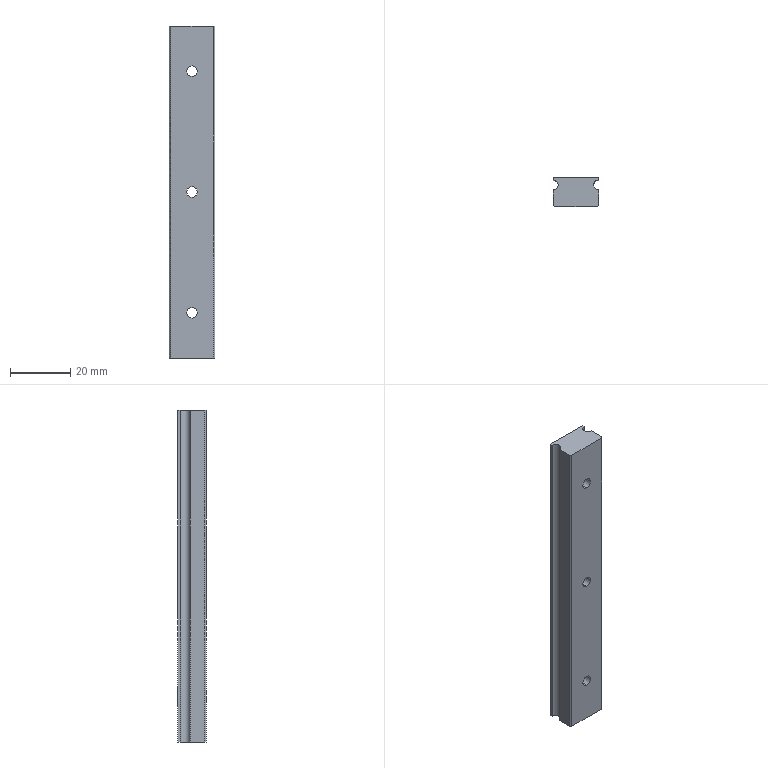Part | SolidWorks | features BaseBody 1 | 1 solid | 28 faces | box 15 x 9.5 x 110 mm | volume 14193 mm3 | cylinder 15 | plane 13 | commonest cylinder face diameters 3.5 x6 6 x6 3.28 x3
STEP:
#1=CARTESIAN_POINT('',(0.,9.5,58.));
#2=VERTEX_POINT('',#1);
#3=CARTESIAN_POINT('',(0.,9.5,52.));
#4=VERTEX_POINT('',#3);
#5=CARTESIAN_POINT('',(0.,9.5,55.));
#6=DIRECTION('',(0.,-1.,0.));
#7=DIRECTION('',(0.,0.,-1.));
#8=AXIS2_PLACEMENT_3D('',#5,#6,#7);
#9=CIRCLE('',#8,3.);
#10=EDGE_CURVE('',#2,#4,#9,.T.);
#11=ORIENTED_EDGE('',*,*,#10,.F.);
#12=CARTESIAN_POINT('',(0.,5.,58.));
#13=VERTEX_POINT('',#12);
#14=CARTESIAN_POINT('',(0.,7.25,58.));
#15=DIRECTION('',(0.,-1.,0.));
#16=VECTOR('',#15,1000.);
#17=LINE('',#14,#16);
#18=EDGE_CURVE('',#2,#13,#17,.T.);
#19=ORIENTED_EDGE('',*,*,#18,.T.);
#20=CARTESIAN_POINT('',(0.,5.,52.));
#21=VERTEX_POINT('',#20);
#22=CARTESIAN_POINT('',(0.,5.,55.));
#23=DIRECTION('',(0.,1.,0.));
#24=DIRECTION('',(0.,0.,-1.));
#25=AXIS2_PLACEMENT_3D('',#22,#23,#24);
#26=CIRCLE('',#25,3.);
#27=EDGE_CURVE('',#21,#13,#26,.T.);
#28=ORIENTED_EDGE('',*,*,#27,.F.);
#29=CARTESIAN_POINT('',(0.,7.25,52.));
#30=DIRECTION('',(0.,-1.,0.));
#31=VECTOR('',#30,1000.);
#32=LINE('',#29,#31);
#33=EDGE_CURVE('',#4,#21,#32,.T.);
#34=ORIENTED_EDGE('',*,*,#33,.F.);
#35=EDGE_LOOP('',(#11,#19,#28,#34));
#36=FACE_OUTER_BOUND('',#35,.T.);
#37=CARTESIAN_POINT('',(0.,7.25,55.));
#38=DIRECTION('',(0.,-1.,0.));
#39=DIRECTION('',(0.,0.,-1.));
#40=AXIS2_PLACEMENT_3D('',#37,#38,#39);
#41=CYLINDRICAL_SURFACE('',#40,3.);
#42=ADVANCED_FACE('',(#36),#41,.F.);
#43=CARTESIAN_POINT('',(0.,9.5,18.));
#44=VERTEX_POINT('',#43);
#45=CARTESIAN_POINT('',(0.,9.5,12.));
#46=VERTEX_POINT('',#45);
#47=CARTESIAN_POINT('',(0.,9.5,15.));
#48=DIRECTION('',(0.,-1.,0.));
#49=DIRECTION('',(0.,0.,-1.));
#50=AXIS2_PLACEMENT_3D('',#47,#48,#49);
#51=CIRCLE('',#50,3.);
#52=EDGE_CURVE('',#44,#46,#51,.T.);
#53=ORIENTED_EDGE('',*,*,#52,.F.);
#54=CARTESIAN_POINT('',(0.,5.,18.));
#55=VERTEX_POINT('',#54);
#56=CARTESIAN_POINT('',(0.,7.25,18.));
#57=DIRECTION('',(0.,-1.,0.));
#58=VECTOR('',#57,1000.);
#59=LINE('',#56,#58);
#60=EDGE_CURVE('',#44,#55,#59,.T.);
#61=ORIENTED_EDGE('',*,*,#60,.T.);
#62=CARTESIAN_POINT('',(0.,5.,12.));
#63=VERTEX_POINT('',#62);
#64=CARTESIAN_POINT('',(0.,5.,15.));
#65=DIRECTION('',(0.,1.,0.));
#66=DIRECTION('',(0.,0.,-1.));
#67=AXIS2_PLACEMENT_3D('',#64,#65,#66);
#68=CIRCLE('',#67,3.);
#69=EDGE_CURVE('',#63,#55,#68,.T.);
#70=ORIENTED_EDGE('',*,*,#69,.F.);
#71=CARTESIAN_POINT('',(0.,7.25,12.));
#72=DIRECTION('',(0.,-1.,0.));
#73=VECTOR('',#72,1000.);
#74=LINE('',#71,#73);
#75=EDGE_CURVE('',#46,#63,#74,.T.);
#76=ORIENTED_EDGE('',*,*,#75,.F.);
#77=EDGE_LOOP('',(#53,#61,#70,#76));
#78=FACE_OUTER_BOUND('',#77,.T.);
#79=CARTESIAN_POINT('',(0.,7.25,15.));
#80=DIRECTION('',(0.,-1.,0.));
#81=DIRECTION('',(0.,0.,-1.));
#82=AXIS2_PLACEMENT_3D('',#79,#80,#81);
#83=CYLINDRICAL_SURFACE('',#82,3.);
#84=ADVANCED_FACE('',(#78),#83,.F.);
#85=CARTESIAN_POINT('',(0.,9.5,98.));
#86=VERTEX_POINT('',#85);
#87=CARTESIAN_POINT('',(0.,9.5,92.));
#88=VERTEX_POINT('',#87);
#89=CARTESIAN_POINT('',(0.,9.5,95.));
#90=DIRECTION('',(0.,-1.,0.));
#91=DIRECTION('',(0.,0.,-1.));
#92=AXIS2_PLACEMENT_3D('',#89,#90,#91);
#93=CIRCLE('',#92,3.);
#94=EDGE_CURVE('',#86,#88,#93,.T.);
#95=ORIENTED_EDGE('',*,*,#94,.F.);
#96=CARTESIAN_POINT('',(0.,5.,98.));
#97=VERTEX_POINT('',#96);
#98=CARTESIAN_POINT('',(0.,7.25,98.));
#99=DIRECTION('',(0.,-1.,0.));
#100=VECTOR('',#99,1000.);
#101=LINE('',#98,#100);
#102=EDGE_CURVE('',#86,#97,#101,.T.);
#103=ORIENTED_EDGE('',*,*,#102,.T.);
#104=CARTESIAN_POINT('',(0.,5.,92.));
#105=VERTEX_POINT('',#104);
#106=CARTESIAN_POINT('',(0.,5.,95.));
#107=DIRECTION('',(0.,1.,0.));
#108=DIRECTION('',(0.,0.,-1.));
#109=AXIS2_PLACEMENT_3D('',#106,#107,#108);
#110=CIRCLE('',#109,3.);
#111=EDGE_CURVE('',#105,#97,#110,.T.);
#112=ORIENTED_EDGE('',*,*,#111,.F.);
#113=CARTESIAN_POINT('',(0.,7.25,92.));
#114=DIRECTION('',(0.,-1.,0.));
#115=VECTOR('',#114,1000.);
#116=LINE('',#113,#115);
#117=EDGE_CURVE('',#88,#105,#116,.T.);
#118=ORIENTED_EDGE('',*,*,#117,.F.);
#119=EDGE_LOOP('',(#95,#103,#112,#118));
#120=FACE_OUTER_BOUND('',#119,.T.);
#121=CARTESIAN_POINT('',(0.,7.25,95.));
#122=DIRECTION('',(0.,-1.,0.));
#123=DIRECTION('',(0.,0.,-1.));
#124=AXIS2_PLACEMENT_3D('',#121,#122,#123);
#125=CYLINDRICAL_SURFACE('',#124,3.);
#126=ADVANCED_FACE('',(#120),#125,.F.);
#127=CARTESIAN_POINT('',(5.86,7.02,110.));
#128=VERTEX_POINT('',#127);
#129=CARTESIAN_POINT('',(7.5,8.66,110.));
#130=VERTEX_POINT('',#129);
#131=CARTESIAN_POINT('',(7.5,7.02,110.));
#132=DIRECTION('',(0.,0.,-1.));
#133=DIRECTION('',(-1.,0.,0.));
#134=AXIS2_PLACEMENT_3D('',#131,#132,#133);
#135=CIRCLE('',#134,1.64);
#136=EDGE_CURVE('',#128,#130,#135,.T.);
#137=ORIENTED_EDGE('',*,*,#136,.F.);
#138=CARTESIAN_POINT('',(5.86,7.02,0.));
#139=VERTEX_POINT('',#138);
#140=CARTESIAN_POINT('',(5.86,7.02,0.));
#141=DIRECTION('',(0.,0.,-1.));
#142=VECTOR('',#141,1000.);
#143=LINE('',#140,#142);
#144=EDGE_CURVE('',#128,#139,#143,.T.);
#145=ORIENTED_EDGE('',*,*,#144,.T.);
#146=CARTESIAN_POINT('',(7.5,8.66,0.));
#147=VERTEX_POINT('',#146);
#148=CARTESIAN_POINT('',(7.5,7.02,0.));
#149=DIRECTION('',(0.,0.,-1.));
#150=DIRECTION('',(-1.,0.,0.));
#151=AXIS2_PLACEMENT_3D('',#148,#149,#150);
#152=CIRCLE('',#151,1.64);
#153=EDGE_CURVE('',#139,#147,#152,.T.);
#154=ORIENTED_EDGE('',*,*,#153,.T.);
#155=CARTESIAN_POINT('',(7.5,8.66,0.));
#156=DIRECTION('',(0.,0.,-1.));
#157=VECTOR('',#156,1000.);
#158=LINE('',#155,#157);
#159=EDGE_CURVE('',#130,#147,#158,.T.);
#160=ORIENTED_EDGE('',*,*,#159,.F.);
#161=EDGE_LOOP('',(#137,#145,#154,#160));
#162=FACE_OUTER_BOUND('',#161,.T.);
#163=CARTESIAN_POINT('',(7.5,7.02,0.));
#164=DIRECTION('',(0.,0.,-1.));
#165=DIRECTION('',(-1.,0.,0.));
#166=AXIS2_PLACEMENT_3D('',#163,#164,#165);
#167=CYLINDRICAL_SURFACE('',#166,1.64);
#168=ADVANCED_FACE('',(#162),#167,.F.);
#169=CARTESIAN_POINT('',(0.,5.,53.25));
#170=VERTEX_POINT('',#169);
#171=CARTESIAN_POINT('',(0.,5.,56.75));
#172=VERTEX_POINT('',#171);
#173=CARTESIAN_POINT('',(0.,5.,55.));
#174=DIRECTION('',(0.,1.,0.));
#175=DIRECTION('',(0.,0.,-1.));
#176=AXIS2_PLACEMENT_3D('',#173,#174,#175);
#177=CIRCLE('',#176,1.75);
#178=EDGE_CURVE('',#170,#172,#177,.T.);
#179=ORIENTED_EDGE('',*,*,#178,.T.);
#180=CARTESIAN_POINT('',(0.,0.,56.75));
#181=VERTEX_POINT('',#180);
#182=CARTESIAN_POINT('',(0.,2.5,56.75));
#183=DIRECTION('',(0.,-1.,0.));
#184=VECTOR('',#183,1000.);
#185=LINE('',#182,#184);
#186=EDGE_CURVE('',#172,#181,#185,.T.);
#187=ORIENTED_EDGE('',*,*,#186,.T.);
#188=CARTESIAN_POINT('',(0.,0.,53.25));
#189=VERTEX_POINT('',#188);
#190=CARTESIAN_POINT('',(0.,0.,55.));
#191=DIRECTION('',(0.,1.,0.));
#192=DIRECTION('',(0.,0.,-1.));
#193=AXIS2_PLACEMENT_3D('',#190,#191,#192);
#194=CIRCLE('',#193,1.75);
#195=EDGE_CURVE('',#189,#181,#194,.T.);
#196=ORIENTED_EDGE('',*,*,#195,.F.);
#197=CARTESIAN_POINT('',(0.,2.5,53.25));
#198=DIRECTION('',(0.,-1.,0.));
#199=VECTOR('',#198,1000.);
#200=LINE('',#197,#199);
#201=EDGE_CURVE('',#170,#189,#200,.T.);
#202=ORIENTED_EDGE('',*,*,#201,.F.);
#203=EDGE_LOOP('',(#179,#187,#196,#202));
#204=FACE_OUTER_BOUND('',#203,.T.);
#205=CARTESIAN_POINT('',(0.,2.5,55.));
#206=DIRECTION('',(0.,-1.,0.));
#207=DIRECTION('',(0.,0.,-1.));
#208=AXIS2_PLACEMENT_3D('',#205,#206,#207);
#209=CYLINDRICAL_SURFACE('',#208,1.75);
#210=ADVANCED_FACE('',(#204),#209,.F.);
#211=CARTESIAN_POINT('',(0.,5.,13.25));
#212=VERTEX_POINT('',#211);
#213=CARTESIAN_POINT('',(0.,5.,16.75));
#214=VERTEX_POINT('',#213);
#215=CARTESIAN_POINT('',(0.,5.,15.));
#216=DIRECTION('',(0.,1.,0.));
#217=DIRECTION('',(0.,0.,-1.));
#218=AXIS2_PLACEMENT_3D('',#215,#216,#217);
#219=CIRCLE('',#218,1.75);
#220=EDGE_CURVE('',#212,#214,#219,.T.);
#221=ORIENTED_EDGE('',*,*,#220,.T.);
#222=CARTESIAN_POINT('',(0.,0.,16.75));
#223=VERTEX_POINT('',#222);
#224=CARTESIAN_POINT('',(0.,2.5,16.75));
#225=DIRECTION('',(0.,-1.,0.));
#226=VECTOR('',#225,1000.);
#227=LINE('',#224,#226);
#228=EDGE_CURVE('',#214,#223,#227,.T.);
#229=ORIENTED_EDGE('',*,*,#228,.T.);
#230=CARTESIAN_POINT('',(0.,0.,13.25));
#231=VERTEX_POINT('',#230);
#232=CARTESIAN_POINT('',(0.,0.,15.));
#233=DIRECTION('',(0.,1.,0.));
#234=DIRECTION('',(0.,0.,-1.));
#235=AXIS2_PLACEMENT_3D('',#232,#233,#234);
#236=CIRCLE('',#235,1.75);
#237=EDGE_CURVE('',#231,#223,#236,.T.);
#238=ORIENTED_EDGE('',*,*,#237,.F.);
#239=CARTESIAN_POINT('',(0.,2.5,13.25));
#240=DIRECTION('',(0.,-1.,0.));
#241=VECTOR('',#240,1000.);
#242=LINE('',#239,#241);
#243=EDGE_CURVE('',#212,#231,#242,.T.);
#244=ORIENTED_EDGE('',*,*,#243,.F.);
#245=EDGE_LOOP('',(#221,#229,#238,#244));
#246=FACE_OUTER_BOUND('',#245,.T.);
#247=CARTESIAN_POINT('',(0.,2.5,15.));
#248=DIRECTION('',(0.,-1.,0.));
#249=DIRECTION('',(0.,0.,-1.));
#250=AXIS2_PLACEMENT_3D('',#247,#248,#249);
#251=CYLINDRICAL_SURFACE('',#250,1.75);
#252=ADVANCED_FACE('',(#246),#251,.F.);
#253=CARTESIAN_POINT('',(0.,5.,93.25));
#254=VERTEX_POINT('',#253);
#255=CARTESIAN_POINT('',(0.,5.,96.75));
#256=VERTEX_POINT('',#255);
#257=CARTESIAN_POINT('',(0.,5.,95.));
#258=DIRECTION('',(0.,1.,0.));
#259=DIRECTION('',(0.,0.,-1.));
#260=AXIS2_PLACEMENT_3D('',#257,#258,#259);
#261=CIRCLE('',#260,1.75);
#262=EDGE_CURVE('',#254,#256,#261,.T.);
#263=ORIENTED_EDGE('',*,*,#262,.T.);
#264=CARTESIAN_POINT('',(0.,0.,96.75));
#265=VERTEX_POINT('',#264);
#266=CARTESIAN_POINT('',(0.,2.5,96.75));
#267=DIRECTION('',(0.,-1.,0.));
#268=VECTOR('',#267,1000.);
#269=LINE('',#266,#268);
#270=EDGE_CURVE('',#256,#265,#269,.T.);
#271=ORIENTED_EDGE('',*,*,#270,.T.);
#272=CARTESIAN_POINT('',(0.,0.,93.25));
#273=VERTEX_POINT('',#272);
#274=CARTESIAN_POINT('',(0.,0.,95.));
#275=DIRECTION('',(0.,1.,0.));
#276=DIRECTION('',(0.,0.,-1.));
#277=AXIS2_PLACEMENT_3D('',#274,#275,#276);
#278=CIRCLE('',#277,1.75);
#279=EDGE_CURVE('',#273,#265,#278,.T.);
#280=ORIENTED_EDGE('',*,*,#279,.F.);
#281=CARTESIAN_POINT('',(0.,2.5,93.25));
#282=DIRECTION('',(0.,-1.,0.));
#283=VECTOR('',#282,1000.);
#284=LINE('',#281,#283);
#285=EDGE_CURVE('',#254,#273,#284,.T.);
#286=ORIENTED_EDGE('',*,*,#285,.F.);
#287=EDGE_LOOP('',(#263,#271,#280,#286));
#288=FACE_OUTER_BOUND('',#287,.T.);
#289=CARTESIAN_POINT('',(0.,2.5,95.));
#290=DIRECTION('',(0.,-1.,0.));
#291=DIRECTION('',(0.,0.,-1.));
#292=AXIS2_PLACEMENT_3D('',#289,#290,#291);
#293=CYLINDRICAL_SURFACE('',#292,1.75);
#294=ADVANCED_FACE('',(#288),#293,.F.);
#295=CARTESIAN_POINT('',(0.,9.5,55.));
#296=DIRECTION('',(0.,-1.,0.));
#297=DIRECTION('',(0.,0.,-1.));
#298=AXIS2_PLACEMENT_3D('',#295,#296,#297);
#299=CIRCLE('',#298,3.);
#300=EDGE_CURVE('',#4,#2,#299,.T.);
#301=ORIENTED_EDGE('',*,*,#300,.T.);
#302=ORIENTED_EDGE('',*,*,#10,.T.);
#303=EDGE_LOOP('',(#301,#302));
#304=FACE_BOUND('',#303,.T.);
#305=CARTESIAN_POINT('',(0.,9.5,15.));
#306=DIRECTION('',(0.,-1.,0.));
#307=DIRECTION('',(0.,0.,-1.));
#308=AXIS2_PLACEMENT_3D('',#305,#306,#307);
#309=CIRCLE('',#308,3.);
#310=EDGE_CURVE('',#46,#44,#309,.T.);
#311=ORIENTED_EDGE('',*,*,#310,.T.);
#312=ORIENTED_EDGE('',*,*,#52,.T.);
#313=EDGE_LOOP('',(#311,#312));
#314=FACE_BOUND('',#313,.T.);
#315=CARTESIAN_POINT('',(0.,9.5,95.));
#316=DIRECTION('',(0.,-1.,0.));
#317=DIRECTION('',(0.,0.,-1.));
#318=AXIS2_PLACEMENT_3D('',#315,#316,#317);
#319=CIRCLE('',#318,3.);
#320=EDGE_CURVE('',#88,#86,#319,.T.);
#321=ORIENTED_EDGE('',*,*,#320,.T.);
#322=ORIENTED_EDGE('',*,*,#94,.T.);
#323=EDGE_LOOP('',(#321,#322));
#324=FACE_BOUND('',#323,.T.);
#325=CARTESIAN_POINT('',(7.5,9.5,0.));
#326=VERTEX_POINT('',#325);
#327=CARTESIAN_POINT('',(-7.5,9.5,0.));
#328=VERTEX_POINT('',#327);
#329=CARTESIAN_POINT('',(-7.5,9.5,0.));
#330=DIRECTION('',(-1.,0.,0.));
#331=VECTOR('',#330,1000.);
#332=LINE('',#329,#331);
#333=EDGE_CURVE('',#326,#328,#332,.T.);
#334=ORIENTED_EDGE('',*,*,#333,.T.);
#335=CARTESIAN_POINT('',(-7.5,9.5,110.));
#336=VERTEX_POINT('',#335);
#337=CARTESIAN_POINT('',(-7.5,9.5,0.));
#338=DIRECTION('',(0.,0.,1.));
#339=VECTOR('',#338,1000.);
#340=LINE('',#337,#339);
#341=EDGE_CURVE('',#328,#336,#340,.T.);
#342=ORIENTED_EDGE('',*,*,#341,.T.);
#343=CARTESIAN_POINT('',(7.5,9.5,110.));
#344=VERTEX_POINT('',#343);
#345=CARTESIAN_POINT('',(-7.5,9.5,110.));
#346=DIRECTION('',(1.,0.,0.));
#347=VECTOR('',#346,1000.);
#348=LINE('',#345,#347);
#349=EDGE_CURVE('',#336,#344,#348,.T.);
#350=ORIENTED_EDGE('',*,*,#349,.T.);
#351=CARTESIAN_POINT('',(7.5,9.5,0.));
#352=DIRECTION('',(0.,0.,-1.));
#353=VECTOR('',#352,1000.);
#354=LINE('',#351,#353);
#355=EDGE_CURVE('',#344,#326,#354,.T.);
#356=ORIENTED_EDGE('',*,*,#355,.T.);
#357=EDGE_LOOP('',(#334,#342,#350,#356));
#358=FACE_OUTER_BOUND('',#357,.T.);
#359=CARTESIAN_POINT('',(-7.5,9.5,0.));
#360=DIRECTION('',(0.,1.,0.));
#361=DIRECTION('',(0.,0.,1.));
#362=AXIS2_PLACEMENT_3D('',#359,#360,#361);
#363=PLANE('',#362);
#364=ADVANCED_FACE('',(#304,#314,#324,#358),#363,.T.);
#365=ORIENTED_EDGE('',*,*,#18,.F.);
#366=ORIENTED_EDGE('',*,*,#300,.F.);
#367=ORIENTED_EDGE('',*,*,#33,.T.);
#368=CARTESIAN_POINT('',(0.,5.,55.));
#369=DIRECTION('',(0.,1.,0.));
#370=DIRECTION('',(0.,0.,-1.));
#371=AXIS2_PLACEMENT_3D('',#368,#369,#370);
#372=CIRCLE('',#371,3.);
#373=EDGE_CURVE('',#13,#21,#372,.T.);
#374=ORIENTED_EDGE('',*,*,#373,.F.);
#375=EDGE_LOOP('',(#365,#366,#367,#374));
#376=FACE_OUTER_BOUND('',#375,.T.);
#377=CARTESIAN_POINT('',(0.,7.25,55.));
#378=DIRECTION('',(0.,-1.,0.));
#379=DIRECTION('',(0.,0.,-1.));
#380=AXIS2_PLACEMENT_3D('',#377,#378,#379);
#381=CYLINDRICAL_SURFACE('',#380,3.);
#382=ADVANCED_FACE('',(#376),#381,.F.);
#383=ORIENTED_EDGE('',*,*,#60,.F.);
#384=ORIENTED_EDGE('',*,*,#310,.F.);
#385=ORIENTED_EDGE('',*,*,#75,.T.);
#386=CARTESIAN_POINT('',(0.,5.,15.));
#387=DIRECTION('',(0.,1.,0.));
#388=DIRECTION('',(0.,0.,-1.));
#389=AXIS2_PLACEMENT_3D('',#386,#387,#388);
#390=CIRCLE('',#389,3.);
#391=EDGE_CURVE('',#55,#63,#390,.T.);
#392=ORIENTED_EDGE('',*,*,#391,.F.);
#393=EDGE_LOOP('',(#383,#384,#385,#392));
#394=FACE_OUTER_BOUND('',#393,.T.);
#395=CARTESIAN_POINT('',(0.,7.25,15.));
#396=DIRECTION('',(0.,-1.,0.));
#397=DIRECTION('',(0.,0.,-1.));
#398=AXIS2_PLACEMENT_3D('',#395,#396,#397);
#399=CYLINDRICAL_SURFACE('',#398,3.);
#400=ADVANCED_FACE('',(#394),#399,.F.);
#401=ORIENTED_EDGE('',*,*,#102,.F.);
#402=ORIENTED_EDGE('',*,*,#320,.F.);
#403=ORIENTED_EDGE('',*,*,#117,.T.);
#404=CARTESIAN_POINT('',(0.,5.,95.));
#405=DIRECTION('',(0.,1.,0.));
#406=DIRECTION('',(0.,0.,-1.));
#407=AXIS2_PLACEMENT_3D('',#404,#405,#406);
#408=CIRCLE('',#407,3.);
#409=EDGE_CURVE('',#97,#105,#408,.T.);
#410=ORIENTED_EDGE('',*,*,#409,.F.);
#411=EDGE_LOOP('',(#401,#402,#403,#410));
#412=FACE_OUTER_BOUND('',#411,.T.);
#413=CARTESIAN_POINT('',(0.,7.25,95.));
#414=DIRECTION('',(0.,-1.,0.));
#415=DIRECTION('',(0.,0.,-1.));
#416=AXIS2_PLACEMENT_3D('',#413,#414,#415);
#417=CYLINDRICAL_SURFACE('',#416,3.);
#418=ADVANCED_FACE('',(#412),#417,.F.);
#419=CARTESIAN_POINT('',(-7.5,8.66,0.));
#420=VERTEX_POINT('',#419);
#421=CARTESIAN_POINT('',(-7.5,8.66,0.));
#422=DIRECTION('',(0.,-1.,0.));
#423=VECTOR('',#422,1000.);
#424=LINE('',#421,#423);
#425=EDGE_CURVE('',#328,#420,#424,.T.);
#426=ORIENTED_EDGE('',*,*,#425,.T.);
#427=CARTESIAN_POINT('',(-7.5,8.66,110.));
#428=VERTEX_POINT('',#427);
#429=CARTESIAN_POINT('',(-7.5,8.66,0.));
#430=DIRECTION('',(0.,0.,1.));
#431=VECTOR('',#430,1000.);
#432=LINE('',#429,#431);
#433=EDGE_CURVE('',#420,#428,#432,.T.);
#434=ORIENTED_EDGE('',*,*,#433,.T.);
#435=CARTESIAN_POINT('',(-7.5,8.66,110.));
#436=DIRECTION('',(0.,1.,0.));
#437=VECTOR('',#436,1000.);
#438=LINE('',#435,#437);
#439=EDGE_CURVE('',#428,#336,#438,.T.);
#440=ORIENTED_EDGE('',*,*,#439,.T.);
#441=ORIENTED_EDGE('',*,*,#341,.F.);
#442=EDGE_LOOP('',(#426,#434,#440,#441));
#443=FACE_OUTER_BOUND('',#442,.T.);
#444=CARTESIAN_POINT('',(-7.5,8.66,0.));
#445=DIRECTION('',(-1.,0.,0.));
#446=DIRECTION('',(0.,0.,1.));
#447=AXIS2_PLACEMENT_3D('',#444,#445,#446);
#448=PLANE('',#447);
#449=ADVANCED_FACE('',(#443),#448,.T.);
#450=ORIENTED_EDGE('',*,*,#333,.F.);
#451=CARTESIAN_POINT('',(7.5,0.,0.));
#452=DIRECTION('',(0.,1.,0.));
#453=VECTOR('',#452,1000.);
#454=LINE('',#451,#453);
#455=EDGE_CURVE('',#147,#326,#454,.T.);
#456=ORIENTED_EDGE('',*,*,#455,.F.);
#457=ORIENTED_EDGE('',*,*,#153,.F.);
#458=CARTESIAN_POINT('',(7.5,5.38,0.));
#459=VERTEX_POINT('',#458);
#460=CARTESIAN_POINT('',(7.5,7.02,0.));
#461=DIRECTION('',(0.,0.,-1.));
#462=DIRECTION('',(-1.,0.,0.));
#463=AXIS2_PLACEMENT_3D('',#460,#461,#462);
#464=CIRCLE('',#463,1.64);
#465=EDGE_CURVE('',#459,#139,#464,.T.);
#466=ORIENTED_EDGE('',*,*,#465,.F.);
#467=CARTESIAN_POINT('',(7.5,0.495,0.));
#468=VERTEX_POINT('',#467);
#469=CARTESIAN_POINT('',(7.5,0.,0.));
#470=DIRECTION('',(0.,1.,0.));
#471=VECTOR('',#470,1000.);
#472=LINE('',#469,#471);
#473=EDGE_CURVE('',#468,#459,#472,.T.);
#474=ORIENTED_EDGE('',*,*,#473,.F.);
#475=CARTESIAN_POINT('',(7.005,0.,0.));
#476=VERTEX_POINT('',#475);
#477=CARTESIAN_POINT('',(7.5,0.495,0.));
#478=DIRECTION('',(0.7071,0.7071,0.));
#479=VECTOR('',#478,1000.);
#480=LINE('',#477,#479);
#481=EDGE_CURVE('',#476,#468,#480,.T.);
#482=ORIENTED_EDGE('',*,*,#481,.F.);
#483=CARTESIAN_POINT('',(-7.005,0.,0.));
#484=VERTEX_POINT('',#483);
#485=CARTESIAN_POINT('',(0.,0.,0.));
#486=DIRECTION('',(1.,0.,0.));
#487=VECTOR('',#486,1000.);
#488=LINE('',#485,#487);
#489=EDGE_CURVE('',#484,#476,#488,.T.);
#490=ORIENTED_EDGE('',*,*,#489,.F.);
#491=CARTESIAN_POINT('',(-7.5,0.495,0.));
#492=VERTEX_POINT('',#491);
#493=CARTESIAN_POINT('',(-7.005,0.,0.));
#494=DIRECTION('',(0.7071,-0.7071,0.));
#495=VECTOR('',#494,1000.);
#496=LINE('',#493,#495);
#497=EDGE_CURVE('',#492,#484,#496,.T.);
#498=ORIENTED_EDGE('',*,*,#497,.F.);
#499=CARTESIAN_POINT('',(-7.5,5.38,0.));
#500=VERTEX_POINT('',#499);
#501=CARTESIAN_POINT('',(-7.5,0.,0.));
#502=DIRECTION('',(0.,-1.,0.));
#503=VECTOR('',#502,1000.);
#504=LINE('',#501,#503);
#505=EDGE_CURVE('',#500,#492,#504,.T.);
#506=ORIENTED_EDGE('',*,*,#505,.F.);
#507=CARTESIAN_POINT('',(-7.5,7.02,0.));
#508=DIRECTION('',(0.,0.,-1.));
#509=DIRECTION('',(-1.,0.,0.));
#510=AXIS2_PLACEMENT_3D('',#507,#508,#509);
#511=CIRCLE('',#510,1.64);
#512=EDGE_CURVE('',#420,#500,#511,.T.);
#513=ORIENTED_EDGE('',*,*,#512,.F.);
#514=ORIENTED_EDGE('',*,*,#425,.F.);
#515=EDGE_LOOP('',(#450,#456,#457,#466,#474,#482,#490,#498,#506,#513,#514));
#516=FACE_OUTER_BOUND('',#515,.T.);
#517=CARTESIAN_POINT('',(0.,0.,0.));
#518=DIRECTION('',(0.,0.,1.));
#519=DIRECTION('',(1.,0.,0.));
#520=AXIS2_PLACEMENT_3D('',#517,#518,#519);
#521=PLANE('',#520);
#522=ADVANCED_FACE('',(#516),#521,.F.);
#523=ORIENTED_EDGE('',*,*,#455,.T.);
#524=ORIENTED_EDGE('',*,*,#355,.F.);
#525=CARTESIAN_POINT('',(7.5,9.5,110.));
#526=DIRECTION('',(0.,-1.,0.));
#527=VECTOR('',#526,1000.);
#528=LINE('',#525,#527);
#529=EDGE_CURVE('',#344,#130,#528,.T.);
#530=ORIENTED_EDGE('',*,*,#529,.T.);
#531=ORIENTED_EDGE('',*,*,#159,.T.);
#532=EDGE_LOOP('',(#523,#524,#530,#531));
#533=FACE_OUTER_BOUND('',#532,.T.);
#534=CARTESIAN_POINT('',(7.5,9.5,0.));
#535=DIRECTION('',(1.,0.,0.));
#536=DIRECTION('',(0.,0.,-1.));
#537=AXIS2_PLACEMENT_3D('',#534,#535,#536);
#538=PLANE('',#537);
#539=ADVANCED_FACE('',(#533),#538,.T.);
#540=CARTESIAN_POINT('',(7.5,5.38,110.));
#541=VERTEX_POINT('',#540);
#542=CARTESIAN_POINT('',(7.5,7.02,110.));
#543=DIRECTION('',(0.,0.,-1.));
#544=DIRECTION('',(-1.,0.,0.));
#545=AXIS2_PLACEMENT_3D('',#542,#543,#544);
#546=CIRCLE('',#545,1.64);
#547=EDGE_CURVE('',#541,#128,#546,.T.);
#548=ORIENTED_EDGE('',*,*,#547,.T.);
#549=ORIENTED_EDGE('',*,*,#136,.T.);
#550=ORIENTED_EDGE('',*,*,#529,.F.);
#551=ORIENTED_EDGE('',*,*,#349,.F.);
#552=ORIENTED_EDGE('',*,*,#439,.F.);
#553=CARTESIAN_POINT('',(-7.5,5.38,110.));
#554=VERTEX_POINT('',#553);
#555=CARTESIAN_POINT('',(-7.5,7.02,110.));
#556=DIRECTION('',(0.,0.,-1.));
#557=DIRECTION('',(-1.,0.,0.));
#558=AXIS2_PLACEMENT_3D('',#555,#556,#557);
#559=CIRCLE('',#558,1.64);
#560=EDGE_CURVE('',#428,#554,#559,.T.);
#561=ORIENTED_EDGE('',*,*,#560,.T.);
#562=CARTESIAN_POINT('',(-7.5,0.495,110.));
#563=VERTEX_POINT('',#562);
#564=CARTESIAN_POINT('',(-7.5,0.,110.));
#565=DIRECTION('',(0.,-1.,0.));
#566=VECTOR('',#565,1000.);
#567=LINE('',#564,#566);
#568=EDGE_CURVE('',#554,#563,#567,.T.);
#569=ORIENTED_EDGE('',*,*,#568,.T.);
#570=CARTESIAN_POINT('',(-7.005,0.,110.));
#571=VERTEX_POINT('',#570);
#572=CARTESIAN_POINT('',(-7.005,0.,110.));
#573=DIRECTION('',(-0.7071,0.7071,0.));
#574=VECTOR('',#573,1000.);
#575=LINE('',#572,#574);
#576=EDGE_CURVE('',#571,#563,#575,.T.);
#577=ORIENTED_EDGE('',*,*,#576,.F.);
#578=CARTESIAN_POINT('',(7.005,0.,110.));
#579=VERTEX_POINT('',#578);
#580=CARTESIAN_POINT('',(0.,0.,110.));
#581=DIRECTION('',(1.,0.,0.));
#582=VECTOR('',#581,1000.);
#583=LINE('',#580,#582);
#584=EDGE_CURVE('',#571,#579,#583,.T.);
#585=ORIENTED_EDGE('',*,*,#584,.T.);
#586=CARTESIAN_POINT('',(7.5,0.495,110.));
#587=VERTEX_POINT('',#586);
#588=CARTESIAN_POINT('',(7.5,0.495,110.));
#589=DIRECTION('',(-0.7071,-0.7071,0.));
#590=VECTOR('',#589,1000.);
#591=LINE('',#588,#590);
#592=EDGE_CURVE('',#587,#579,#591,.T.);
#593=ORIENTED_EDGE('',*,*,#592,.F.);
#594=CARTESIAN_POINT('',(7.5,0.,110.));
#595=DIRECTION('',(0.,1.,0.));
#596=VECTOR('',#595,1000.);
#597=LINE('',#594,#596);
#598=EDGE_CURVE('',#587,#541,#597,.T.);
#599=ORIENTED_EDGE('',*,*,#598,.T.);
#600=EDGE_LOOP('',(#548,#549,#550,#551,#552,#561,#569,#577,#585,#593,#599));
#601=FACE_OUTER_BOUND('',#600,.T.);
#602=CARTESIAN_POINT('',(0.,0.,110.));
#603=DIRECTION('',(0.,0.,1.));
#604=DIRECTION('',(1.,0.,0.));
#605=AXIS2_PLACEMENT_3D('',#602,#603,#604);
#606=PLANE('',#605);
#607=ADVANCED_FACE('',(#601),#606,.T.);
#608=ORIENTED_EDGE('',*,*,#178,.F.);
#609=CARTESIAN_POINT('',(0.,5.,55.));
#610=DIRECTION('',(0.,1.,0.));
#611=DIRECTION('',(0.,0.,-1.));
#612=AXIS2_PLACEMENT_3D('',#609,#610,#611);
#613=CIRCLE('',#612,1.75);
#614=EDGE_CURVE('',#172,#170,#613,.T.);
#615=ORIENTED_EDGE('',*,*,#614,.F.);
#616=EDGE_LOOP('',(#608,#615));
#617=FACE_BOUND('',#616,.T.);
#618=ORIENTED_EDGE('',*,*,#27,.T.);
#619=ORIENTED_EDGE('',*,*,#373,.T.);
#620=EDGE_LOOP('',(#618,#619));
#621=FACE_OUTER_BOUND('',#620,.T.);
#622=CARTESIAN_POINT('',(0.,5.,52.625));
#623=DIRECTION('',(0.,-1.,0.));
#624=DIRECTION('',(0.,0.,-1.));
#625=AXIS2_PLACEMENT_3D('',#622,#623,#624);
#626=PLANE('',#625);
#627=ADVANCED_FACE('',(#617,#621),#626,.F.);
#628=ORIENTED_EDGE('',*,*,#220,.F.);
#629=CARTESIAN_POINT('',(0.,5.,15.));
#630=DIRECTION('',(0.,1.,0.));
#631=DIRECTION('',(0.,0.,-1.));
#632=AXIS2_PLACEMENT_3D('',#629,#630,#631);
#633=CIRCLE('',#632,1.75);
#634=EDGE_CURVE('',#214,#212,#633,.T.);
#635=ORIENTED_EDGE('',*,*,#634,.F.);
#636=EDGE_LOOP('',(#628,#635));
#637=FACE_BOUND('',#636,.T.);
#638=ORIENTED_EDGE('',*,*,#69,.T.);
#639=ORIENTED_EDGE('',*,*,#391,.T.);
#640=EDGE_LOOP('',(#638,#639));
#641=FACE_OUTER_BOUND('',#640,.T.);
#642=CARTESIAN_POINT('',(0.,5.,12.625));
#643=DIRECTION('',(0.,-1.,0.));
#644=DIRECTION('',(0.,0.,-1.));
#645=AXIS2_PLACEMENT_3D('',#642,#643,#644);
#646=PLANE('',#645);
#647=ADVANCED_FACE('',(#637,#641),#646,.F.);
#648=ORIENTED_EDGE('',*,*,#262,.F.);
#649=CARTESIAN_POINT('',(0.,5.,95.));
#650=DIRECTION('',(0.,1.,0.));
#651=DIRECTION('',(0.,0.,-1.));
#652=AXIS2_PLACEMENT_3D('',#649,#650,#651);
#653=CIRCLE('',#652,1.75);
#654=EDGE_CURVE('',#256,#254,#653,.T.);
#655=ORIENTED_EDGE('',*,*,#654,.F.);
#656=EDGE_LOOP('',(#648,#655));
#657=FACE_BOUND('',#656,.T.);
#658=ORIENTED_EDGE('',*,*,#111,.T.);
#659=ORIENTED_EDGE('',*,*,#409,.T.);
#660=EDGE_LOOP('',(#658,#659));
#661=FACE_OUTER_BOUND('',#660,.T.);
#662=CARTESIAN_POINT('',(0.,5.,92.625));
#663=DIRECTION('',(0.,-1.,0.));
#664=DIRECTION('',(0.,0.,-1.));
#665=AXIS2_PLACEMENT_3D('',#662,#663,#664);
#666=PLANE('',#665);
#667=ADVANCED_FACE('',(#657,#661),#666,.F.);
#668=ORIENTED_EDGE('',*,*,#433,.F.);
#669=ORIENTED_EDGE('',*,*,#512,.T.);
#670=CARTESIAN_POINT('',(-7.5,5.38,0.));
#671=DIRECTION('',(0.,0.,-1.));
#672=VECTOR('',#671,1000.);
#673=LINE('',#670,#672);
#674=EDGE_CURVE('',#554,#500,#673,.T.);
#675=ORIENTED_EDGE('',*,*,#674,.F.);
#676=ORIENTED_EDGE('',*,*,#560,.F.);
#677=EDGE_LOOP('',(#668,#669,#675,#676));
#678=FACE_OUTER_BOUND('',#677,.T.);
#679=CARTESIAN_POINT('',(-7.5,7.02,0.));
#680=DIRECTION('',(0.,0.,-1.));
#681=DIRECTION('',(-1.,0.,0.));
#682=AXIS2_PLACEMENT_3D('',#679,#680,#681);
#683=CYLINDRICAL_SURFACE('',#682,1.64);
#684=ADVANCED_FACE('',(#678),#683,.F.);
#685=ORIENTED_EDGE('',*,*,#144,.F.);
#686=ORIENTED_EDGE('',*,*,#547,.F.);
#687=CARTESIAN_POINT('',(7.5,5.38,0.));
#688=DIRECTION('',(0.,0.,1.));
#689=VECTOR('',#688,1000.);
#690=LINE('',#687,#689);
#691=EDGE_CURVE('',#459,#541,#690,.T.);
#692=ORIENTED_EDGE('',*,*,#691,.F.);
#693=ORIENTED_EDGE('',*,*,#465,.T.);
#694=EDGE_LOOP('',(#685,#686,#692,#693));
#695=FACE_OUTER_BOUND('',#694,.T.);
#696=CARTESIAN_POINT('',(7.5,7.02,0.));
#697=DIRECTION('',(0.,0.,-1.));
#698=DIRECTION('',(-1.,0.,0.));
#699=AXIS2_PLACEMENT_3D('',#696,#697,#698);
#700=CYLINDRICAL_SURFACE('',#699,1.64);
#701=ADVANCED_FACE('',(#695),#700,.F.);
#702=ORIENTED_EDGE('',*,*,#473,.T.);
#703=ORIENTED_EDGE('',*,*,#691,.T.);
#704=ORIENTED_EDGE('',*,*,#598,.F.);
#705=CARTESIAN_POINT('',(7.5,0.495,0.));
#706=DIRECTION('',(0.,0.,-1.));
#707=VECTOR('',#706,1000.);
#708=LINE('',#705,#707);
#709=EDGE_CURVE('',#587,#468,#708,.T.);
#710=ORIENTED_EDGE('',*,*,#709,.T.);
#711=EDGE_LOOP('',(#702,#703,#704,#710));
#712=FACE_OUTER_BOUND('',#711,.T.);
#713=CARTESIAN_POINT('',(7.5,5.38,0.));
#714=DIRECTION('',(1.,0.,0.));
#715=DIRECTION('',(0.,0.,-1.));
#716=AXIS2_PLACEMENT_3D('',#713,#714,#715);
#717=PLANE('',#716);
#718=ADVANCED_FACE('',(#712),#717,.T.);
#719=ORIENTED_EDGE('',*,*,#195,.T.);
#720=CARTESIAN_POINT('',(0.,0.,55.));
#721=DIRECTION('',(0.,1.,0.));
#722=DIRECTION('',(0.,0.,-1.));
#723=AXIS2_PLACEMENT_3D('',#720,#721,#722);
#724=CIRCLE('',#723,1.75);
#725=EDGE_CURVE('',#181,#189,#724,.T.);
#726=ORIENTED_EDGE('',*,*,#725,.T.);
#727=EDGE_LOOP('',(#719,#726));
#728=FACE_BOUND('',#727,.T.);
#729=ORIENTED_EDGE('',*,*,#237,.T.);
#730=CARTESIAN_POINT('',(0.,0.,15.));
#731=DIRECTION('',(0.,1.,0.));
#732=DIRECTION('',(0.,0.,-1.));
#733=AXIS2_PLACEMENT_3D('',#730,#731,#732);
#734=CIRCLE('',#733,1.75);
#735=EDGE_CURVE('',#223,#231,#734,.T.);
#736=ORIENTED_EDGE('',*,*,#735,.T.);
#737=EDGE_LOOP('',(#729,#736));
#738=FACE_BOUND('',#737,.T.);
#739=ORIENTED_EDGE('',*,*,#279,.T.);
#740=CARTESIAN_POINT('',(0.,0.,95.));
#741=DIRECTION('',(0.,1.,0.));
#742=DIRECTION('',(0.,0.,-1.));
#743=AXIS2_PLACEMENT_3D('',#740,#741,#742);
#744=CIRCLE('',#743,1.75);
#745=EDGE_CURVE('',#265,#273,#744,.T.);
#746=ORIENTED_EDGE('',*,*,#745,.T.);
#747=EDGE_LOOP('',(#739,#746));
#748=FACE_BOUND('',#747,.T.);
#749=ORIENTED_EDGE('',*,*,#489,.T.);
#750=CARTESIAN_POINT('',(7.005,0.,0.));
#751=DIRECTION('',(0.,0.,1.));
#752=VECTOR('',#751,1000.);
#753=LINE('',#750,#752);
#754=EDGE_CURVE('',#476,#579,#753,.T.);
#755=ORIENTED_EDGE('',*,*,#754,.T.);
#756=ORIENTED_EDGE('',*,*,#584,.F.);
#757=CARTESIAN_POINT('',(-7.005,0.,0.));
#758=DIRECTION('',(0.,0.,-1.));
#759=VECTOR('',#758,1000.);
#760=LINE('',#757,#759);
#761=EDGE_CURVE('',#571,#484,#760,.T.);
#762=ORIENTED_EDGE('',*,*,#761,.T.);
#763=EDGE_LOOP('',(#749,#755,#756,#762));
#764=FACE_OUTER_BOUND('',#763,.T.);
#765=CARTESIAN_POINT('',(7.005,0.,0.));
#766=DIRECTION('',(0.,-1.,0.));
#767=DIRECTION('',(0.,0.,-1.));
#768=AXIS2_PLACEMENT_3D('',#765,#766,#767);
#769=PLANE('',#768);
#770=ADVANCED_FACE('',(#728,#738,#748,#764),#769,.T.);
#771=ORIENTED_EDGE('',*,*,#505,.T.);
#772=CARTESIAN_POINT('',(-7.5,0.495,0.));
#773=DIRECTION('',(0.,0.,1.));
#774=VECTOR('',#773,1000.);
#775=LINE('',#772,#774);
#776=EDGE_CURVE('',#492,#563,#775,.T.);
#777=ORIENTED_EDGE('',*,*,#776,.T.);
#778=ORIENTED_EDGE('',*,*,#568,.F.);
#779=ORIENTED_EDGE('',*,*,#674,.T.);
#780=EDGE_LOOP('',(#771,#777,#778,#779));
#781=FACE_OUTER_BOUND('',#780,.T.);
#782=CARTESIAN_POINT('',(-7.5,0.495,0.));
#783=DIRECTION('',(-1.,0.,0.));
#784=DIRECTION('',(0.,0.,1.));
#785=AXIS2_PLACEMENT_3D('',#782,#783,#784);
#786=PLANE('',#785);
#787=ADVANCED_FACE('',(#781),#786,.T.);
#788=ORIENTED_EDGE('',*,*,#186,.F.);
#789=ORIENTED_EDGE('',*,*,#614,.T.);
#790=ORIENTED_EDGE('',*,*,#201,.T.);
#791=ORIENTED_EDGE('',*,*,#725,.F.);
#792=EDGE_LOOP('',(#788,#789,#790,#791));
#793=FACE_OUTER_BOUND('',#792,.T.);
#794=CARTESIAN_POINT('',(0.,2.5,55.));
#795=DIRECTION('',(0.,-1.,0.));
#796=DIRECTION('',(0.,0.,-1.));
#797=AXIS2_PLACEMENT_3D('',#794,#795,#796);
#798=CYLINDRICAL_SURFACE('',#797,1.75);
#799=ADVANCED_FACE('',(#793),#798,.F.);
#800=ORIENTED_EDGE('',*,*,#228,.F.);
#801=ORIENTED_EDGE('',*,*,#634,.T.);
#802=ORIENTED_EDGE('',*,*,#243,.T.);
#803=ORIENTED_EDGE('',*,*,#735,.F.);
#804=EDGE_LOOP('',(#800,#801,#802,#803));
#805=FACE_OUTER_BOUND('',#804,.T.);
#806=CARTESIAN_POINT('',(0.,2.5,15.));
#807=DIRECTION('',(0.,-1.,0.));
#808=DIRECTION('',(0.,0.,-1.));
#809=AXIS2_PLACEMENT_3D('',#806,#807,#808);
#810=CYLINDRICAL_SURFACE('',#809,1.75);
#811=ADVANCED_FACE('',(#805),#810,.F.);
#812=ORIENTED_EDGE('',*,*,#270,.F.);
#813=ORIENTED_EDGE('',*,*,#654,.T.);
#814=ORIENTED_EDGE('',*,*,#285,.T.);
#815=ORIENTED_EDGE('',*,*,#745,.F.);
#816=EDGE_LOOP('',(#812,#813,#814,#815));
#817=FACE_OUTER_BOUND('',#816,.T.);
#818=CARTESIAN_POINT('',(0.,2.5,95.));
#819=DIRECTION('',(0.,-1.,0.));
#820=DIRECTION('',(0.,0.,-1.));
#821=AXIS2_PLACEMENT_3D('',#818,#819,#820);
#822=CYLINDRICAL_SURFACE('',#821,1.75);
#823=ADVANCED_FACE('',(#817),#822,.F.);
#824=ORIENTED_EDGE('',*,*,#481,.T.);
#825=ORIENTED_EDGE('',*,*,#709,.F.);
#826=ORIENTED_EDGE('',*,*,#592,.T.);
#827=ORIENTED_EDGE('',*,*,#754,.F.);
#828=EDGE_LOOP('',(#824,#825,#826,#827));
#829=FACE_OUTER_BOUND('',#828,.T.);
#830=CARTESIAN_POINT('',(7.5,0.495,0.));
#831=DIRECTION('',(0.7071,-0.7071,0.));
#832=DIRECTION('',(0.7071,0.7071,0.));
#833=AXIS2_PLACEMENT_3D('',#830,#831,#832);
#834=PLANE('',#833);
#835=ADVANCED_FACE('',(#829),#834,.T.);
#836=ORIENTED_EDGE('',*,*,#497,.T.);
#837=ORIENTED_EDGE('',*,*,#761,.F.);
#838=ORIENTED_EDGE('',*,*,#576,.T.);
#839=ORIENTED_EDGE('',*,*,#776,.F.);
#840=EDGE_LOOP('',(#836,#837,#838,#839));
#841=FACE_OUTER_BOUND('',#840,.T.);
#842=CARTESIAN_POINT('',(-7.005,0.,0.));
#843=DIRECTION('',(-0.7071,-0.7071,0.));
#844=DIRECTION('',(0.7071,-0.7071,0.));
#845=AXIS2_PLACEMENT_3D('',#842,#843,#844);
#846=PLANE('',#845);
#847=ADVANCED_FACE('',(#841),#846,.T.);
#848=CLOSED_SHELL('',(#42,#84,#126,#168,#210,#252,#294,#364,#382,#400,#418,#449,#522,#539,#607,#627,#647,#667,#684,#701,#718,#770,#787,#799,#811,#823,#835,#847));
#849=MANIFOLD_SOLID_BREP('',#848);
#850=CARTESIAN_POINT('',(0.,0.,0.));
#851=DIRECTION('',(0.,0.,1.));
#852=DIRECTION('',(1.,0.,0.));
#853=AXIS2_PLACEMENT_3D('',#850,#851,#852);
#854=(LENGTH_UNIT()NAMED_UNIT(*)SI_UNIT(.MILLI.,.METRE.));
#855=UNCERTAINTY_MEASURE_WITH_UNIT(LENGTH_MEASURE(0.00001),#854,'','');
#856=(NAMED_UNIT(*)PLANE_ANGLE_UNIT()SI_UNIT($,.RADIAN.));
#857=(NAMED_UNIT(*)SI_UNIT($,.STERADIAN.)SOLID_ANGLE_UNIT());
#858=(GEOMETRIC_REPRESENTATION_CONTEXT(3)GLOBAL_UNCERTAINTY_ASSIGNED_CONTEXT((#855))GLOBAL_UNIT_ASSIGNED_CONTEXT((#854,#856,#857))REPRESENTATION_CONTEXT('',''));
#859=ADVANCED_BREP_SHAPE_REPRESENTATION('',(#849,#853),#858);